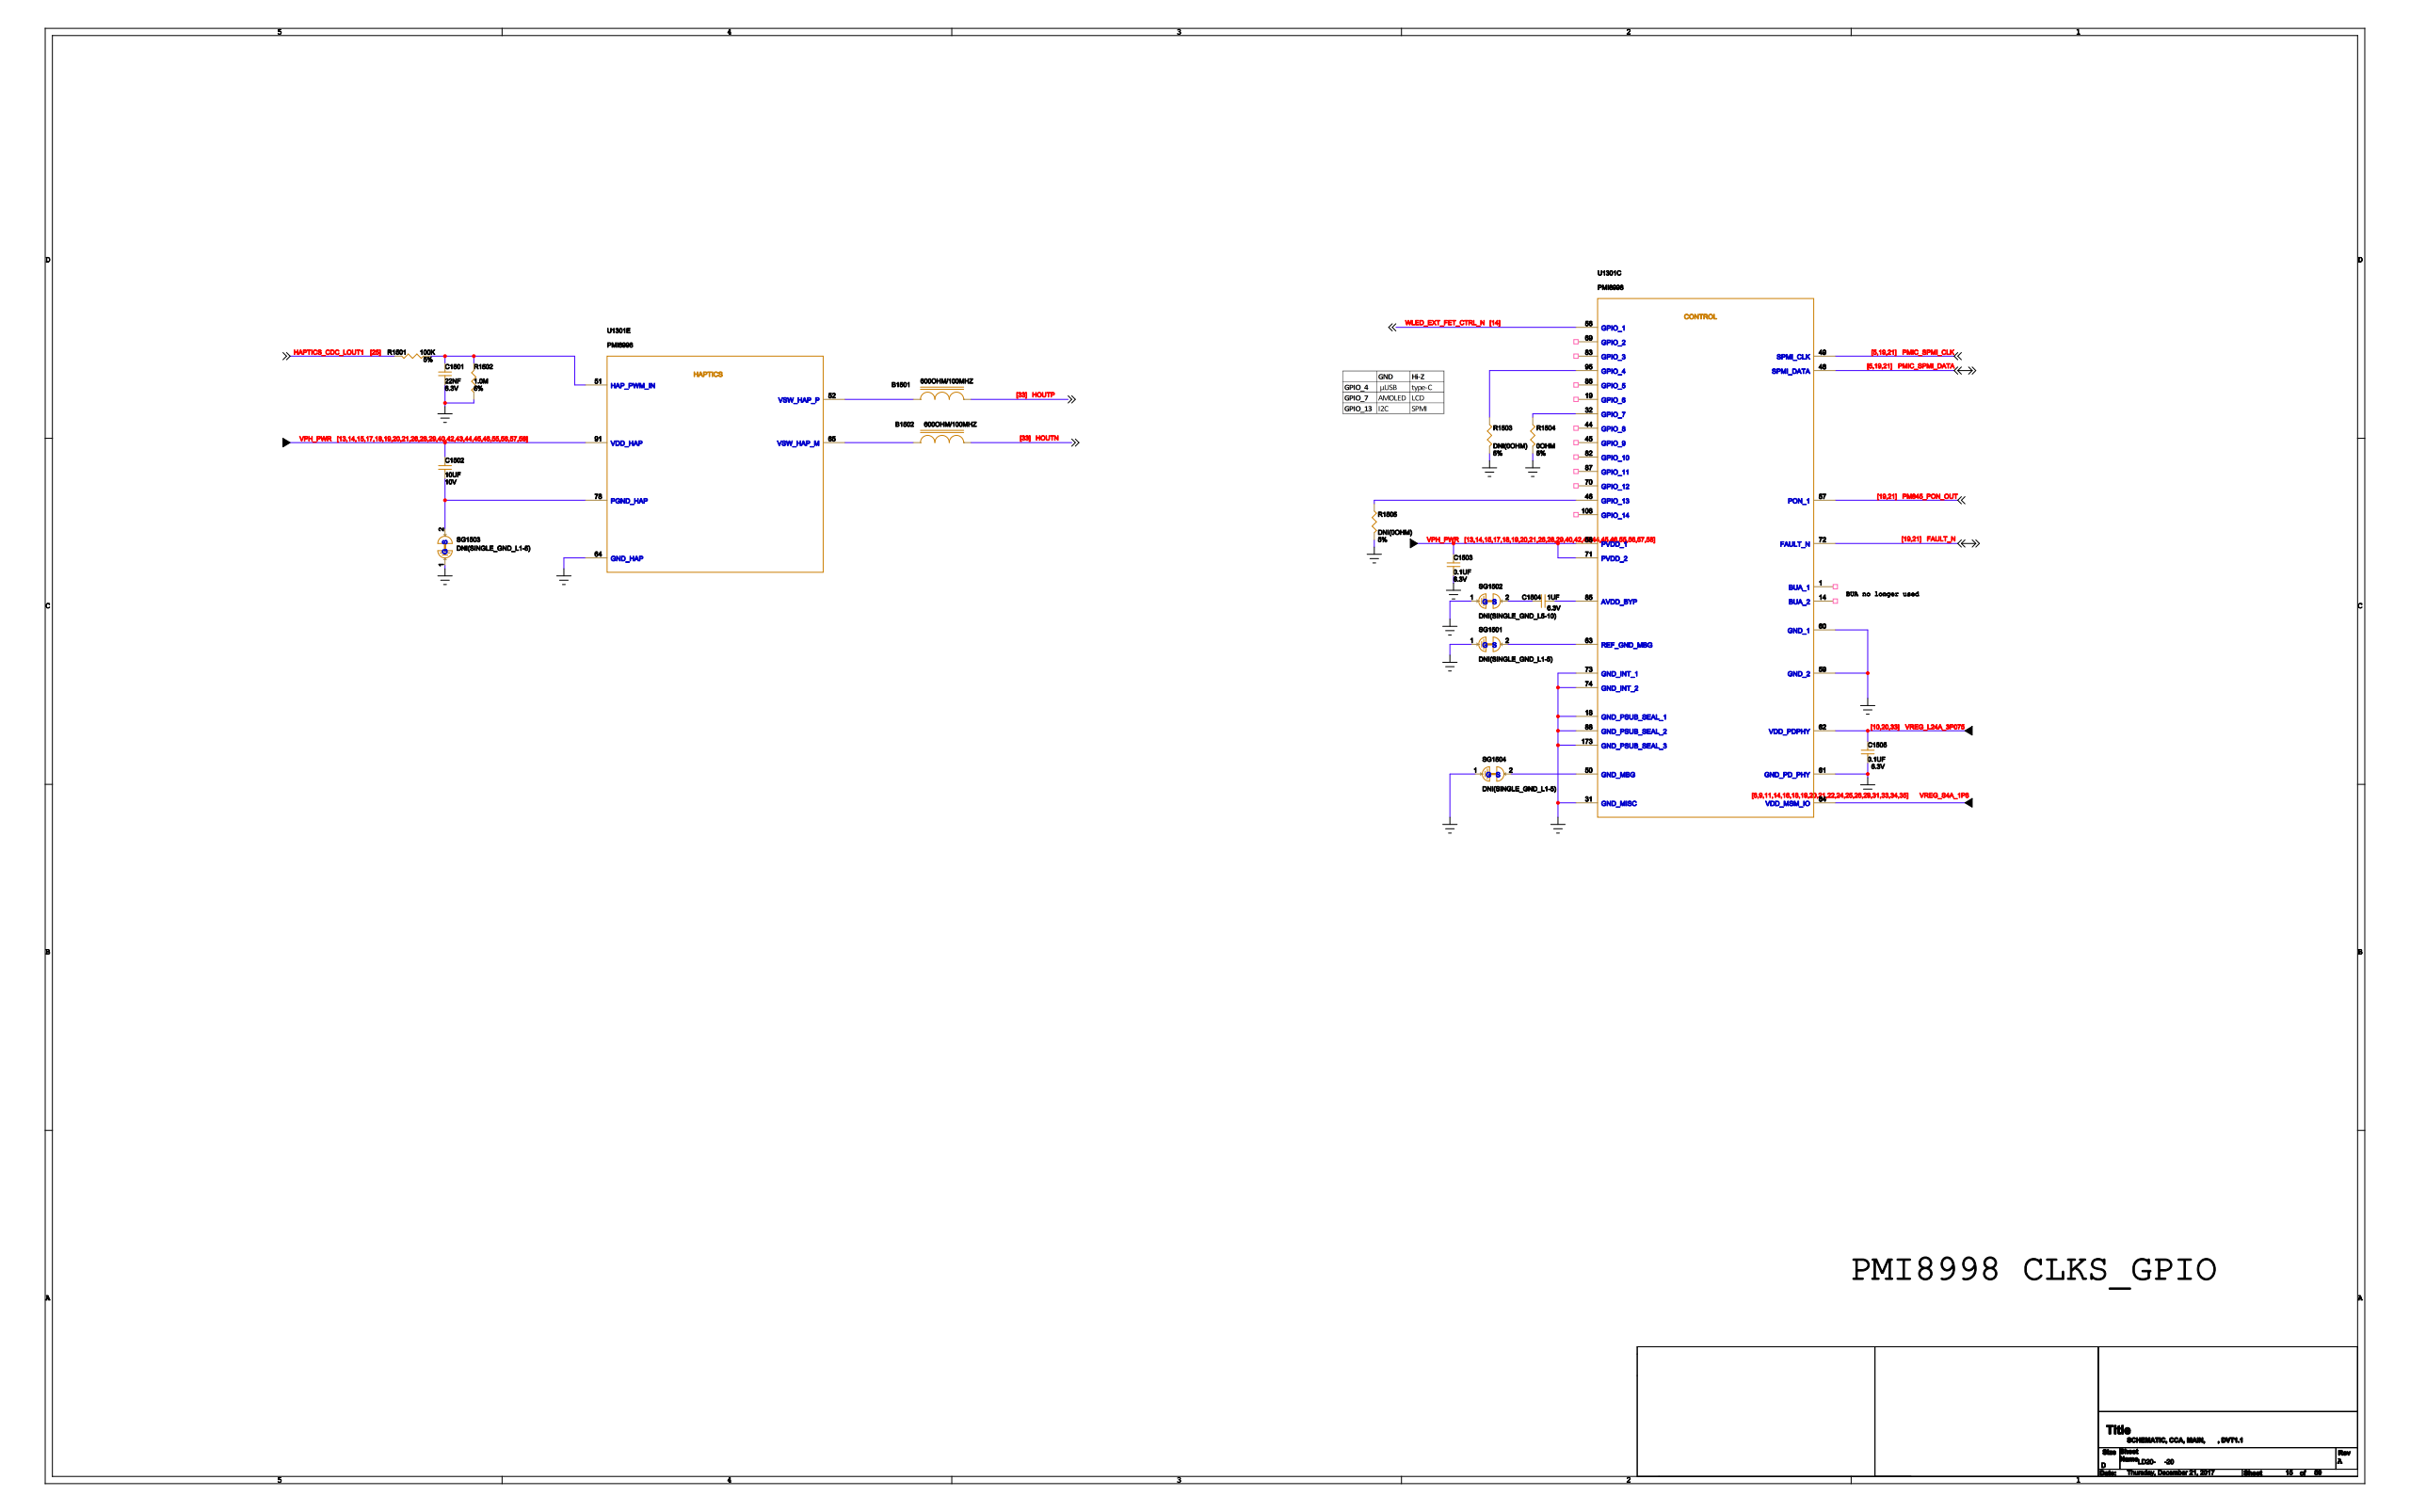Circuit board | Cadence Allegro | 1520 parts | 1149 nets | one sheet of the schematic
Parts on this sheet (reference | value | footprint):
B1501 | 600OHM/100MHZ | 2P0402R
B1502 | 600OHM/100MHZ | 2P0402R
C1501 | 22NF | 2P0201R
C1502 | 10UF | 2P0402RV1
C1503 | 0.1UF | 2P0201R
C1504 | 1UF | 2P0201R
C1505 | 0.1UF | 2P0201R
R1501 | 100K | 2P0201R
R1502 | 1.0M | 2P0201R
R1503 | DNI(0OHM) | 2P0201R_DNI
R1504 | 0OHM | 2P0201R
R1505 | DNI(0OHM) | 2P0201R_DNI
SG1501 | DNI(SINGLE_GND_L1-5) | GND_L1-5
SG1502 | DNI(SINGLE_GND_L5-10) | GND_L5-10
SG1503 | DNI(SINGLE_GND_L1-5) | GND_L1-5
SG1504 | DNI(SINGLE_GND_L1-5) | GND_L1-5
U1301 | PMI8998 | 182PGA229X212B157
Nets of these parts (net: part-pin ...):
GND: C1501-2 C1503-2 C1505-2 R1502-2 R1503-1 R1504-1 R1505-1 SG1501-1 SG1502-1 SG1503-1 SG1504-1 U1301-15 U1301-18 U1301-31 U1301-43 U1301-59 U1301-60 U1301-61 U1301-64 U1301-73 U1301-74 U1301-88 U1301-173
VREG_S4A_1P8: U1301-84
N34047702: SG1501-2 U1301-63
N34047006: C1502-2 SG1503-2 U1301-78
N35147483: SG1504-2 U1301-50
N34908548: C1504-1 SG1502-2
VPH_PWR: C1502-1 C1503-1 U1301-2 U1301-9 U1301-22 U1301-42 U1301-58 U1301-71 U1301-91
VREG_L24A_3P075: C1505-1 U1301-62
HAPTICS_CDC_LOUT1: R1501-1
N34047097: B1501-1 U1301-52
HOUTP: B1501-2
N34047101: B1502-1 U1301-65
HOUTN: B1502-2
N34047561: C1504-2 U1301-85
N34046840: C1501-1 R1501-2 R1502-1 U1301-51
N34047288: R1504-2 U1301-32
WLED_EXT_FET_CTRL_N: U1301-56
N34047250: R1503-2 U1301-95
N34047328: R1505-2 U1301-46
PMIC_SPMI_DATA: U1301-48
PMIC_SPMI_CLK: U1301-49
FAULT_N: U1301-72
PM845_PON_OUT: U1301-57